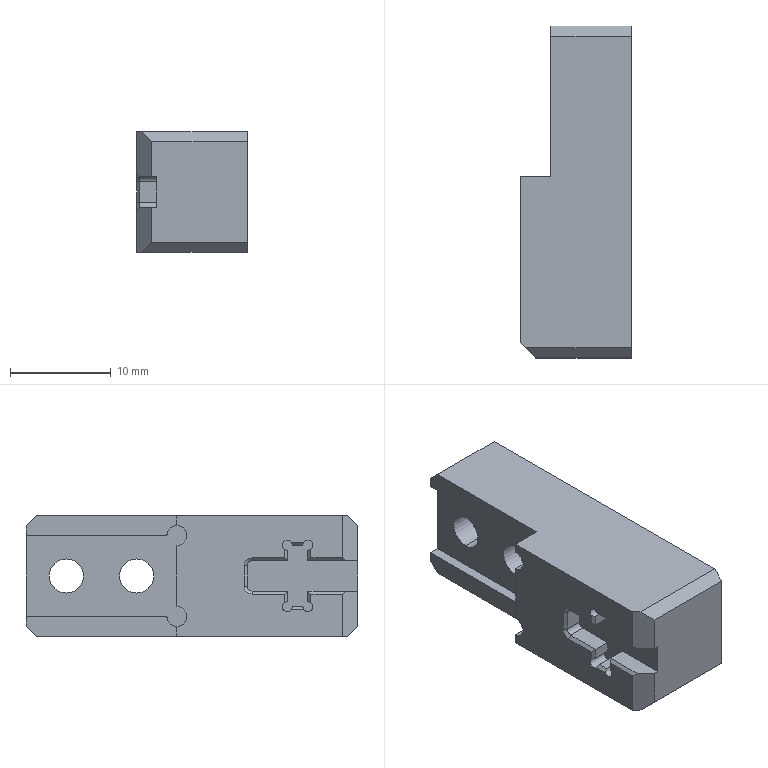Part | STEP file | PN_0051 | 1 solid | 61 faces | box 11 x 33 x 12 mm | volume 3442 mm3 | plane 43 | cylinder 16 | cone 2 | commonest cylinder face diameters 1 x8 2 x4 3.4 x4